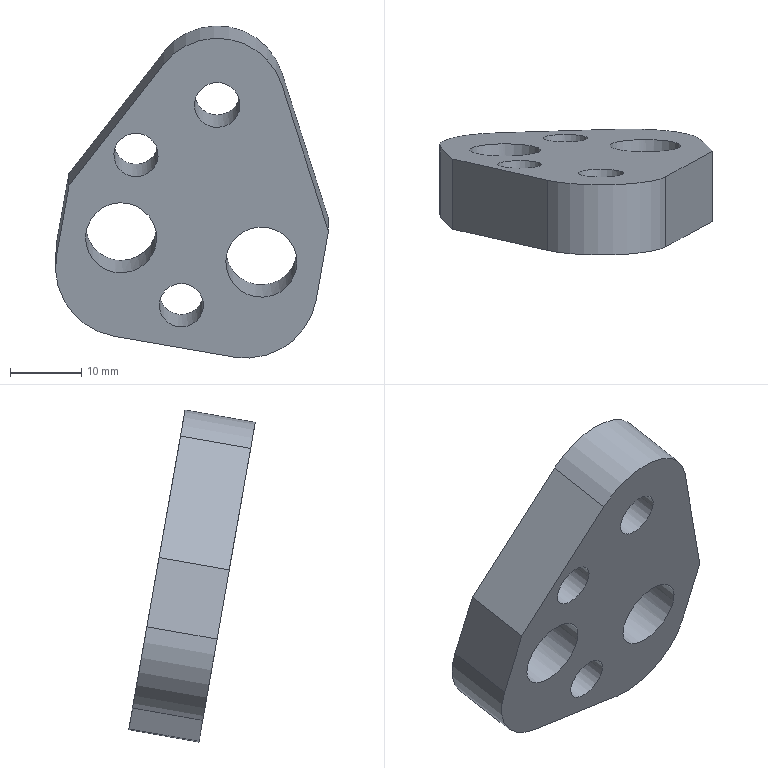Part | NX | features solid 2 | 1 solid | 15 faces | box 38.326 x 17.766 x 46.64 mm | volume 10309 mm3 | cylinder 8 | plane 7 | commonest cylinder face diameters 6.2 x2 10 x2 20 x2 6.4 x1 19 x1
STEP:
#1=CARTESIAN_POINT('',(526.611,650.238,-8.916));
#2=VERTEX_POINT('',#1);
#3=CARTESIAN_POINT('',(534.722,652.25,-20.324));
#4=VERTEX_POINT('',#3);
#5=CARTESIAN_POINT('',(536.459,650.54,-10.626));
#6=DIRECTION('',(0.,-0.9848,-0.1736));
#7=DIRECTION('',(-0.1736,0.171,-0.9698));
#8=AXIS2_PLACEMENT_3D('',#5,#6,#7);
#9=CIRCLE('',#8,10.);
#10=EDGE_CURVE('',#2,#4,#9,.T.);
#11=ORIENTED_EDGE('',*,*,#10,.F.);
#12=CARTESIAN_POINT('',(526.611,660.086,-7.179));
#13=VERTEX_POINT('',#12);
#14=CARTESIAN_POINT('',(526.611,655.162,-8.048));
#15=DIRECTION('',(0.,-0.9848,-0.1736));
#16=VECTOR('',#15,1000.);
#17=LINE('',#14,#16);
#18=EDGE_CURVE('',#13,#2,#17,.T.);
#19=ORIENTED_EDGE('',*,*,#18,.F.);
#20=CARTESIAN_POINT('',(534.722,662.098,-18.588));
#21=VERTEX_POINT('',#20);
#22=CARTESIAN_POINT('',(536.459,660.388,-8.889));
#23=DIRECTION('',(0.,-0.9848,-0.1736));
#24=DIRECTION('',(0.,0.1736,-0.9848));
#25=AXIS2_PLACEMENT_3D('',#22,#23,#24);
#26=CIRCLE('',#25,10.);
#27=EDGE_CURVE('',#13,#21,#26,.T.);
#28=ORIENTED_EDGE('',*,*,#27,.T.);
#29=CARTESIAN_POINT('',(534.722,657.174,-19.456));
#30=DIRECTION('',(0.,-0.9848,-0.1736));
#31=VECTOR('',#30,1000.);
#32=LINE('',#29,#31);
#33=EDGE_CURVE('',#21,#4,#32,.T.);
#34=ORIENTED_EDGE('',*,*,#33,.T.);
#35=EDGE_LOOP('',(#11,#19,#28,#34));
#36=FACE_BOUND('',#35,.T.);
#37=CARTESIAN_POINT('',(536.459,655.464,-9.758));
#38=DIRECTION('',(0.,-0.9848,-0.1736));
#39=DIRECTION('',(-0.1736,0.171,-0.9698));
#40=AXIS2_PLACEMENT_3D('',#37,#38,#39);
#41=CYLINDRICAL_SURFACE('',#40,10.);
#42=ADVANCED_FACE('',(#36),#41,.T.);
#43=CARTESIAN_POINT('',(551.464,652.763,-23.232));
#44=VERTEX_POINT('',#43);
#45=CARTESIAN_POINT('',(551.464,652.763,-23.232));
#46=DIRECTION('',(-0.9848,-0.03015,0.171));
#47=VECTOR('',#46,1000.);
#48=LINE('',#45,#47);
#49=EDGE_CURVE('',#44,#4,#48,.T.);
#50=ORIENTED_EDGE('',*,*,#49,.T.);
#51=ORIENTED_EDGE('',*,*,#33,.F.);
#52=CARTESIAN_POINT('',(551.464,662.611,-21.495));
#53=VERTEX_POINT('',#52);
#54=CARTESIAN_POINT('',(534.722,662.098,-18.588));
#55=DIRECTION('',(-0.9848,-0.03015,0.171));
#56=VECTOR('',#55,1000.);
#57=LINE('',#54,#56);
#58=EDGE_CURVE('',#53,#21,#57,.T.);
#59=ORIENTED_EDGE('',*,*,#58,.F.);
#60=CARTESIAN_POINT('',(551.464,657.687,-22.363));
#61=DIRECTION('',(0.,-0.9848,-0.1736));
#62=VECTOR('',#61,1000.);
#63=LINE('',#60,#62);
#64=EDGE_CURVE('',#53,#44,#63,.T.);
#65=ORIENTED_EDGE('',*,*,#64,.T.);
#66=EDGE_LOOP('',(#50,#51,#59,#65));
#67=FACE_BOUND('',#66,.T.);
#68=CARTESIAN_POINT('',(551.464,657.687,-22.363));
#69=DIRECTION('',(0.1736,-0.171,0.9698));
#70=DIRECTION('',(0.,-0.9848,-0.1736));
#71=AXIS2_PLACEMENT_3D('',#68,#69,#70);
#72=PLANE('',#71);
#73=ADVANCED_FACE('',(#67),#72,.F.);
#74=CARTESIAN_POINT('',(563.049,651.354,-15.243));
#75=VERTEX_POINT('',#74);
#76=CARTESIAN_POINT('',(553.201,651.053,-13.533));
#77=DIRECTION('',(0.,-0.9848,-0.1736));
#78=DIRECTION('',(-0.1736,0.171,-0.9698));
#79=AXIS2_PLACEMENT_3D('',#76,#77,#78);
#80=CIRCLE('',#79,10.);
#81=EDGE_CURVE('',#44,#75,#80,.T.);
#82=ORIENTED_EDGE('',*,*,#81,.F.);
#83=ORIENTED_EDGE('',*,*,#64,.F.);
#84=CARTESIAN_POINT('',(563.049,661.202,-13.507));
#85=VERTEX_POINT('',#84);
#86=CARTESIAN_POINT('',(553.201,660.901,-11.797));
#87=DIRECTION('',(0.,-0.9848,-0.1736));
#88=DIRECTION('',(0.,0.1736,-0.9848));
#89=AXIS2_PLACEMENT_3D('',#86,#87,#88);
#90=CIRCLE('',#89,10.);
#91=EDGE_CURVE('',#53,#85,#90,.T.);
#92=ORIENTED_EDGE('',*,*,#91,.T.);
#93=CARTESIAN_POINT('',(563.049,656.278,-14.375));
#94=DIRECTION('',(0.,-0.9848,-0.1736));
#95=VECTOR('',#94,1000.);
#96=LINE('',#93,#95);
#97=EDGE_CURVE('',#85,#75,#96,.T.);
#98=ORIENTED_EDGE('',*,*,#97,.T.);
#99=EDGE_LOOP('',(#82,#83,#92,#98));
#100=FACE_BOUND('',#99,.T.);
#101=CARTESIAN_POINT('',(553.201,655.977,-12.665));
#102=DIRECTION('',(0.,-0.9848,-0.1736));
#103=DIRECTION('',(-0.1736,0.171,-0.9698));
#104=AXIS2_PLACEMENT_3D('',#101,#102,#103);
#105=CYLINDRICAL_SURFACE('',#104,10.);
#106=ADVANCED_FACE('',(#100),#105,.T.);
#107=CARTESIAN_POINT('',(564.785,649.644,-5.545));
#108=VERTEX_POINT('',#107);
#109=CARTESIAN_POINT('',(564.785,649.644,-5.545));
#110=DIRECTION('',(-0.1736,0.171,-0.9698));
#111=VECTOR('',#110,1000.);
#112=LINE('',#109,#111);
#113=EDGE_CURVE('',#108,#75,#112,.T.);
#114=ORIENTED_EDGE('',*,*,#113,.T.);
#115=ORIENTED_EDGE('',*,*,#97,.F.);
#116=CARTESIAN_POINT('',(564.785,659.492,-3.808));
#117=VERTEX_POINT('',#116);
#118=CARTESIAN_POINT('',(563.049,661.202,-13.507));
#119=DIRECTION('',(-0.1736,0.171,-0.9698));
#120=VECTOR('',#119,1000.);
#121=LINE('',#118,#120);
#122=EDGE_CURVE('',#117,#85,#121,.T.);
#123=ORIENTED_EDGE('',*,*,#122,.F.);
#124=CARTESIAN_POINT('',(564.785,654.568,-4.676));
#125=DIRECTION('',(0.,-0.9848,-0.1736));
#126=VECTOR('',#125,1000.);
#127=LINE('',#124,#126);
#128=EDGE_CURVE('',#117,#108,#127,.T.);
#129=ORIENTED_EDGE('',*,*,#128,.T.);
#130=EDGE_LOOP('',(#114,#115,#123,#129));
#131=FACE_BOUND('',#130,.T.);
#132=CARTESIAN_POINT('',(564.785,654.568,-4.676));
#133=DIRECTION('',(-0.9848,-0.03015,0.171));
#134=DIRECTION('',(0.1736,-0.171,0.9698));
#135=AXIS2_PLACEMENT_3D('',#132,#133,#134);
#136=PLANE('',#135);
#137=ADVANCED_FACE('',(#131),#136,.F.);
#138=CARTESIAN_POINT('',(558.233,646.026,14.973));
#139=VERTEX_POINT('',#138);
#140=CARTESIAN_POINT('',(558.233,646.026,14.973));
#141=DIRECTION('',(0.3,0.1657,-0.9395));
#142=VECTOR('',#141,1000.);
#143=LINE('',#140,#142);
#144=EDGE_CURVE('',#139,#108,#143,.T.);
#145=ORIENTED_EDGE('',*,*,#144,.T.);
#146=ORIENTED_EDGE('',*,*,#128,.F.);
#147=CARTESIAN_POINT('',(558.233,655.874,16.71));
#148=VERTEX_POINT('',#147);
#149=CARTESIAN_POINT('',(563.713,658.9,-0.4492));
#150=DIRECTION('',(0.3,0.1657,-0.9395));
#151=VECTOR('',#150,1000.);
#152=LINE('',#149,#151);
#153=EDGE_CURVE('',#148,#117,#152,.T.);
#154=ORIENTED_EDGE('',*,*,#153,.F.);
#155=CARTESIAN_POINT('',(558.233,650.95,15.841));
#156=DIRECTION('',(0.,-0.9848,-0.1736));
#157=VECTOR('',#156,1000.);
#158=LINE('',#155,#157);
#159=EDGE_CURVE('',#148,#139,#158,.T.);
#160=ORIENTED_EDGE('',*,*,#159,.T.);
#161=EDGE_LOOP('',(#145,#146,#154,#160));
#162=FACE_BOUND('',#161,.T.);
#163=CARTESIAN_POINT('',(558.233,650.95,15.841));
#164=DIRECTION('',(-0.9539,0.05209,-0.2954));
#165=DIRECTION('',(-0.3,-0.1657,0.9395));
#166=AXIS2_PLACEMENT_3D('',#163,#164,#165);
#167=PLANE('',#166);
#168=ADVANCED_FACE('',(#162),#167,.F.);
#169=CARTESIAN_POINT('',(541.63,645.518,17.856));
#170=VERTEX_POINT('',#169);
#171=CARTESIAN_POINT('',(549.171,646.521,12.167));
#172=DIRECTION('',(0.,-0.9848,-0.1736));
#173=DIRECTION('',(-0.1736,0.171,-0.9698));
#174=AXIS2_PLACEMENT_3D('',#171,#172,#173);
#175=CIRCLE('',#174,9.5);
#176=EDGE_CURVE('',#139,#170,#175,.T.);
#177=ORIENTED_EDGE('',*,*,#176,.F.);
#178=ORIENTED_EDGE('',*,*,#159,.F.);
#179=CARTESIAN_POINT('',(541.63,655.366,19.593));
#180=VERTEX_POINT('',#179);
#181=CARTESIAN_POINT('',(549.171,656.369,13.903));
#182=DIRECTION('',(0.,-0.9848,-0.1736));
#183=DIRECTION('',(0.,0.1736,-0.9848));
#184=AXIS2_PLACEMENT_3D('',#181,#182,#183);
#185=CIRCLE('',#184,9.5);
#186=EDGE_CURVE('',#148,#180,#185,.T.);
#187=ORIENTED_EDGE('',*,*,#186,.T.);
#188=CARTESIAN_POINT('',(541.63,650.442,18.725));
#189=DIRECTION('',(0.,-0.9848,-0.1736));
#190=VECTOR('',#189,1000.);
#191=LINE('',#188,#190);
#192=EDGE_CURVE('',#180,#170,#191,.T.);
#193=ORIENTED_EDGE('',*,*,#192,.T.);
#194=EDGE_LOOP('',(#177,#178,#187,#193));
#195=FACE_BOUND('',#194,.T.);
#196=CARTESIAN_POINT('',(549.171,651.445,13.035));
#197=DIRECTION('',(0.,-0.9848,-0.1736));
#198=DIRECTION('',(-0.1736,0.171,-0.9698));
#199=AXIS2_PLACEMENT_3D('',#196,#197,#198);
#200=CYLINDRICAL_SURFACE('',#199,9.5);
#201=ADVANCED_FACE('',(#195),#200,.T.);
#202=CARTESIAN_POINT('',(528.347,648.528,0.7827));
#203=VERTEX_POINT('',#202);
#204=CARTESIAN_POINT('',(541.63,645.518,17.856));
#205=DIRECTION('',(-0.6082,0.1378,-0.7818));
#206=VECTOR('',#205,1000.);
#207=LINE('',#204,#206);
#208=EDGE_CURVE('',#170,#203,#207,.T.);
#209=ORIENTED_EDGE('',*,*,#208,.F.);
#210=ORIENTED_EDGE('',*,*,#192,.F.);
#211=CARTESIAN_POINT('',(528.347,658.376,2.519));
#212=VERTEX_POINT('',#211);
#213=CARTESIAN_POINT('',(525.755,658.964,-0.8133));
#214=DIRECTION('',(-0.6082,0.1378,-0.7818));
#215=VECTOR('',#214,1000.);
#216=LINE('',#213,#215);
#217=EDGE_CURVE('',#180,#212,#216,.T.);
#218=ORIENTED_EDGE('',*,*,#217,.T.);
#219=CARTESIAN_POINT('',(528.347,653.452,1.651));
#220=DIRECTION('',(0.,-0.9848,-0.1736));
#221=VECTOR('',#220,1000.);
#222=LINE('',#219,#221);
#223=EDGE_CURVE('',#212,#203,#222,.T.);
#224=ORIENTED_EDGE('',*,*,#223,.T.);
#225=EDGE_LOOP('',(#209,#210,#218,#224));
#226=FACE_BOUND('',#225,.T.);
#227=CARTESIAN_POINT('',(541.63,650.442,18.725));
#228=DIRECTION('',(-0.7938,-0.1056,0.5989));
#229=DIRECTION('',(0.6082,-0.1378,0.7818));
#230=AXIS2_PLACEMENT_3D('',#227,#228,#229);
#231=PLANE('',#230);
#232=ADVANCED_FACE('',(#226),#231,.T.);
#233=CARTESIAN_POINT('',(528.347,648.528,0.7827));
#234=DIRECTION('',(-0.1736,0.171,-0.9698));
#235=VECTOR('',#234,1000.);
#236=LINE('',#233,#235);
#237=EDGE_CURVE('',#203,#2,#236,.T.);
#238=ORIENTED_EDGE('',*,*,#237,.F.);
#239=ORIENTED_EDGE('',*,*,#223,.F.);
#240=CARTESIAN_POINT('',(526.611,660.086,-7.179));
#241=DIRECTION('',(-0.1736,0.171,-0.9698));
#242=VECTOR('',#241,1000.);
#243=LINE('',#240,#242);
#244=EDGE_CURVE('',#212,#13,#243,.T.);
#245=ORIENTED_EDGE('',*,*,#244,.T.);
#246=ORIENTED_EDGE('',*,*,#18,.T.);
#247=EDGE_LOOP('',(#238,#239,#245,#246));
#248=FACE_BOUND('',#247,.T.);
#249=CARTESIAN_POINT('',(528.347,653.452,1.651));
#250=DIRECTION('',(-0.9848,-0.03015,0.171));
#251=DIRECTION('',(0.1736,-0.171,0.9698));
#252=AXIS2_PLACEMENT_3D('',#249,#250,#251);
#253=PLANE('',#252);
#254=ADVANCED_FACE('',(#248),#253,.T.);
#255=CARTESIAN_POINT('',(555.372,661.13,-13.098));
#256=VERTEX_POINT('',#255);
#257=CARTESIAN_POINT('',(555.372,660.262,-8.174));
#258=DIRECTION('',(0.,-0.9848,-0.1736));
#259=DIRECTION('',(0.,0.1736,-0.9848));
#260=AXIS2_PLACEMENT_3D('',#257,#258,#259);
#261=CIRCLE('',#260,5.);
#262=EDGE_CURVE('',#256,#256,#261,.T.);
#263=ORIENTED_EDGE('',*,*,#262,.T.);
#264=EDGE_LOOP('',(#263));
#265=FACE_BOUND('',#264,.T.);
#266=CARTESIAN_POINT('',(535.676,660.527,-9.678));
#267=VERTEX_POINT('',#266);
#268=CARTESIAN_POINT('',(535.676,659.659,-4.753));
#269=DIRECTION('',(0.,-0.9848,-0.1736));
#270=DIRECTION('',(0.,0.1736,-0.9848));
#271=AXIS2_PLACEMENT_3D('',#268,#269,#270);
#272=CIRCLE('',#271,5.);
#273=EDGE_CURVE('',#267,#267,#272,.T.);
#274=ORIENTED_EDGE('',*,*,#273,.T.);
#275=EDGE_LOOP('',(#274));
#276=FACE_BOUND('',#275,.T.);
#277=CARTESIAN_POINT('',(549.171,656.925,10.752));
#278=VERTEX_POINT('',#277);
#279=CARTESIAN_POINT('',(549.171,656.369,13.903));
#280=DIRECTION('',(0.,-0.9848,-0.1736));
#281=DIRECTION('',(0.,0.1736,-0.9848));
#282=AXIS2_PLACEMENT_3D('',#279,#280,#281);
#283=CIRCLE('',#282,3.2);
#284=EDGE_CURVE('',#278,#278,#283,.T.);
#285=ORIENTED_EDGE('',*,*,#284,.T.);
#286=EDGE_LOOP('',(#285));
#287=FACE_BOUND('',#286,.T.);
#288=CARTESIAN_POINT('',(537.76,658.145,3.832));
#289=VERTEX_POINT('',#288);
#290=CARTESIAN_POINT('',(537.76,657.607,6.885));
#291=DIRECTION('',(0.,-0.9848,-0.1736));
#292=DIRECTION('',(0.,0.1736,-0.9848));
#293=AXIS2_PLACEMENT_3D('',#290,#291,#292);
#294=CIRCLE('',#293,3.1);
#295=EDGE_CURVE('',#289,#289,#294,.T.);
#296=ORIENTED_EDGE('',*,*,#295,.T.);
#297=EDGE_LOOP('',(#296));
#298=FACE_BOUND('',#297,.T.);
#299=CARTESIAN_POINT('',(544.135,661.867,-17.275));
#300=VERTEX_POINT('',#299);
#301=CARTESIAN_POINT('',(544.135,661.328,-14.222));
#302=DIRECTION('',(0.,-0.9848,-0.1736));
#303=DIRECTION('',(0.,0.1736,-0.9848));
#304=AXIS2_PLACEMENT_3D('',#301,#302,#303);
#305=CIRCLE('',#304,3.1);
#306=EDGE_CURVE('',#300,#300,#305,.T.);
#307=ORIENTED_EDGE('',*,*,#306,.T.);
#308=EDGE_LOOP('',(#307));
#309=FACE_BOUND('',#308,.T.);
#310=ORIENTED_EDGE('',*,*,#27,.F.);
#311=ORIENTED_EDGE('',*,*,#244,.F.);
#312=ORIENTED_EDGE('',*,*,#217,.F.);
#313=ORIENTED_EDGE('',*,*,#186,.F.);
#314=ORIENTED_EDGE('',*,*,#153,.T.);
#315=ORIENTED_EDGE('',*,*,#122,.T.);
#316=ORIENTED_EDGE('',*,*,#91,.F.);
#317=ORIENTED_EDGE('',*,*,#58,.T.);
#318=EDGE_LOOP('',(#310,#311,#312,#313,#314,#315,#316,#317));
#319=FACE_BOUND('',#318,.T.);
#320=CARTESIAN_POINT('',(536.459,660.388,-8.889));
#321=DIRECTION('',(0.,-0.9848,-0.1736));
#322=DIRECTION('',(-0.1736,0.171,-0.9698));
#323=AXIS2_PLACEMENT_3D('',#320,#321,#322);
#324=PLANE('',#323);
#325=ADVANCED_FACE('',(#265,#276,#287,#298,#309,#319),#324,.F.);
#326=CARTESIAN_POINT('',(554.504,651.269,-14.759));
#327=VERTEX_POINT('',#326);
#328=CARTESIAN_POINT('',(555.372,650.414,-9.91));
#329=DIRECTION('',(0.,-0.9848,-0.1736));
#330=DIRECTION('',(-0.1736,0.171,-0.9698));
#331=AXIS2_PLACEMENT_3D('',#328,#329,#330);
#332=CIRCLE('',#331,5.);
#333=EDGE_CURVE('',#327,#327,#332,.T.);
#334=ORIENTED_EDGE('',*,*,#333,.F.);
#335=EDGE_LOOP('',(#334));
#336=FACE_BOUND('',#335,.T.);
#337=CARTESIAN_POINT('',(534.808,650.666,-11.339));
#338=VERTEX_POINT('',#337);
#339=CARTESIAN_POINT('',(535.676,649.811,-6.49));
#340=DIRECTION('',(0.,-0.9848,-0.1736));
#341=DIRECTION('',(-0.1736,0.171,-0.9698));
#342=AXIS2_PLACEMENT_3D('',#339,#340,#341);
#343=CIRCLE('',#342,5.);
#344=EDGE_CURVE('',#338,#338,#343,.T.);
#345=ORIENTED_EDGE('',*,*,#344,.F.);
#346=EDGE_LOOP('',(#345));
#347=FACE_BOUND('',#346,.T.);
#348=CARTESIAN_POINT('',(548.615,647.068,9.063));
#349=VERTEX_POINT('',#348);
#350=CARTESIAN_POINT('',(549.171,646.521,12.167));
#351=DIRECTION('',(0.,-0.9848,-0.1736));
#352=DIRECTION('',(-0.1736,0.171,-0.9698));
#353=AXIS2_PLACEMENT_3D('',#350,#351,#352);
#354=CIRCLE('',#353,3.2);
#355=EDGE_CURVE('',#349,#349,#354,.T.);
#356=ORIENTED_EDGE('',*,*,#355,.F.);
#357=EDGE_LOOP('',(#356));
#358=FACE_BOUND('',#357,.T.);
#359=CARTESIAN_POINT('',(537.222,648.289,2.142));
#360=VERTEX_POINT('',#359);
#361=CARTESIAN_POINT('',(537.76,647.758,5.148));
#362=DIRECTION('',(0.,-0.9848,-0.1736));
#363=DIRECTION('',(-0.1736,0.171,-0.9698));
#364=AXIS2_PLACEMENT_3D('',#361,#362,#363);
#365=CIRCLE('',#364,3.1);
#366=EDGE_CURVE('',#360,#360,#365,.T.);
#367=ORIENTED_EDGE('',*,*,#366,.F.);
#368=EDGE_LOOP('',(#367));
#369=FACE_BOUND('',#368,.T.);
#370=CARTESIAN_POINT('',(543.597,652.01,-18.965));
#371=VERTEX_POINT('',#370);
#372=CARTESIAN_POINT('',(544.135,651.48,-15.959));
#373=DIRECTION('',(0.,-0.9848,-0.1736));
#374=DIRECTION('',(-0.1736,0.171,-0.9698));
#375=AXIS2_PLACEMENT_3D('',#372,#373,#374);
#376=CIRCLE('',#375,3.1);
#377=EDGE_CURVE('',#371,#371,#376,.T.);
#378=ORIENTED_EDGE('',*,*,#377,.F.);
#379=EDGE_LOOP('',(#378));
#380=FACE_BOUND('',#379,.T.);
#381=ORIENTED_EDGE('',*,*,#10,.T.);
#382=ORIENTED_EDGE('',*,*,#49,.F.);
#383=ORIENTED_EDGE('',*,*,#81,.T.);
#384=ORIENTED_EDGE('',*,*,#113,.F.);
#385=ORIENTED_EDGE('',*,*,#144,.F.);
#386=ORIENTED_EDGE('',*,*,#176,.T.);
#387=ORIENTED_EDGE('',*,*,#208,.T.);
#388=ORIENTED_EDGE('',*,*,#237,.T.);
#389=EDGE_LOOP('',(#381,#382,#383,#384,#385,#386,#387,#388));
#390=FACE_BOUND('',#389,.T.);
#391=CARTESIAN_POINT('',(536.459,650.54,-10.626));
#392=DIRECTION('',(0.,-0.9848,-0.1736));
#393=DIRECTION('',(-0.1736,0.171,-0.9698));
#394=AXIS2_PLACEMENT_3D('',#391,#392,#393);
#395=PLANE('',#394);
#396=ADVANCED_FACE('',(#336,#347,#358,#369,#380,#390),#395,.T.);
#397=ORIENTED_EDGE('',*,*,#377,.T.);
#398=EDGE_LOOP('',(#397));
#399=FACE_BOUND('',#398,.T.);
#400=ORIENTED_EDGE('',*,*,#306,.F.);
#401=EDGE_LOOP('',(#400));
#402=FACE_BOUND('',#401,.T.);
#403=CARTESIAN_POINT('',(544.135,656.404,-15.091));
#404=DIRECTION('',(0.,-0.9848,-0.1736));
#405=DIRECTION('',(-0.1736,0.171,-0.9698));
#406=AXIS2_PLACEMENT_3D('',#403,#404,#405);
#407=CYLINDRICAL_SURFACE('',#406,3.1);
#408=ADVANCED_FACE('',(#399,#402),#407,.F.);
#409=ORIENTED_EDGE('',*,*,#366,.T.);
#410=EDGE_LOOP('',(#409));
#411=FACE_BOUND('',#410,.T.);
#412=ORIENTED_EDGE('',*,*,#295,.F.);
#413=EDGE_LOOP('',(#412));
#414=FACE_BOUND('',#413,.T.);
#415=CARTESIAN_POINT('',(537.76,652.683,6.016));
#416=DIRECTION('',(0.,-0.9848,-0.1736));
#417=DIRECTION('',(-0.1736,0.171,-0.9698));
#418=AXIS2_PLACEMENT_3D('',#415,#416,#417);
#419=CYLINDRICAL_SURFACE('',#418,3.1);
#420=ADVANCED_FACE('',(#411,#414),#419,.F.);
#421=ORIENTED_EDGE('',*,*,#355,.T.);
#422=EDGE_LOOP('',(#421));
#423=FACE_BOUND('',#422,.T.);
#424=ORIENTED_EDGE('',*,*,#284,.F.);
#425=EDGE_LOOP('',(#424));
#426=FACE_BOUND('',#425,.T.);
#427=CARTESIAN_POINT('',(549.171,651.445,13.035));
#428=DIRECTION('',(0.,-0.9848,-0.1736));
#429=DIRECTION('',(-0.1736,0.171,-0.9698));
#430=AXIS2_PLACEMENT_3D('',#427,#428,#429);
#431=CYLINDRICAL_SURFACE('',#430,3.2);
#432=ADVANCED_FACE('',(#423,#426),#431,.F.);
#433=ORIENTED_EDGE('',*,*,#344,.T.);
#434=EDGE_LOOP('',(#433));
#435=FACE_BOUND('',#434,.T.);
#436=ORIENTED_EDGE('',*,*,#273,.F.);
#437=EDGE_LOOP('',(#436));
#438=FACE_BOUND('',#437,.T.);
#439=CARTESIAN_POINT('',(535.676,654.735,-5.622));
#440=DIRECTION('',(0.,-0.9848,-0.1736));
#441=DIRECTION('',(-0.1736,0.171,-0.9698));
#442=AXIS2_PLACEMENT_3D('',#439,#440,#441);
#443=CYLINDRICAL_SURFACE('',#442,5.);
#444=ADVANCED_FACE('',(#435,#438),#443,.F.);
#445=ORIENTED_EDGE('',*,*,#333,.T.);
#446=EDGE_LOOP('',(#445));
#447=FACE_BOUND('',#446,.T.);
#448=ORIENTED_EDGE('',*,*,#262,.F.);
#449=EDGE_LOOP('',(#448));
#450=FACE_BOUND('',#449,.T.);
#451=CARTESIAN_POINT('',(555.372,655.338,-9.042));
#452=DIRECTION('',(0.,-0.9848,-0.1736));
#453=DIRECTION('',(-0.1736,0.171,-0.9698));
#454=AXIS2_PLACEMENT_3D('',#451,#452,#453);
#455=CYLINDRICAL_SURFACE('',#454,5.);
#456=ADVANCED_FACE('',(#447,#450),#455,.F.);
#457=CLOSED_SHELL('',(#42,#73,#106,#137,#168,#201,#232,#254,#325,#396,#408,#420,#432,#444,#456));
#458=MANIFOLD_SOLID_BREP('',#457);
#459=(LENGTH_UNIT()NAMED_UNIT(*)SI_UNIT(.MILLI.,.METRE.));
#460=UNCERTAINTY_MEASURE_WITH_UNIT(LENGTH_MEASURE(0.00001),#459,'','');
#461=(NAMED_UNIT(*)PLANE_ANGLE_UNIT()SI_UNIT($,.RADIAN.));
#462=(NAMED_UNIT(*)SI_UNIT($,.STERADIAN.)SOLID_ANGLE_UNIT());
#463=(GEOMETRIC_REPRESENTATION_CONTEXT(3)GLOBAL_UNCERTAINTY_ASSIGNED_CONTEXT((#460))GLOBAL_UNIT_ASSIGNED_CONTEXT((#459,#461,#462))REPRESENTATION_CONTEXT('',''));
#464=ADVANCED_BREP_SHAPE_REPRESENTATION('',(#458),#463);